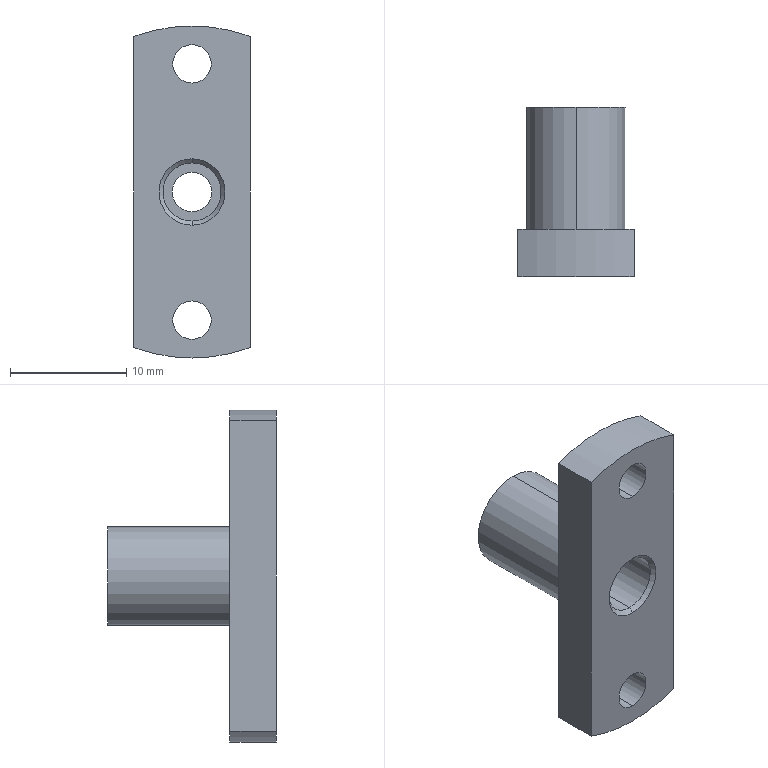Part | NX | features BREP 1 | 1 solid | 23 faces | box 10 x 14.5 x 28.5 mm | volume 1361 mm3 | cylinder 13 | plane 6 | cone 4 | commonest cylinder face diameters 3.3 x4 28.5 x3 3.4 x2 5 x2 8.5 x2
STEP:
#1=CARTESIAN_POINT('',(0.,0.35,2.5));
#2=VERTEX_POINT('',#1);
#3=CARTESIAN_POINT('',(0.,0.,2.85));
#4=VERTEX_POINT('',#3);
#5=CARTESIAN_POINT('',(0.,0.35,2.5));
#6=DIRECTION('',(0.,-0.7071,0.7071));
#7=VECTOR('',#6,1000.);
#8=LINE('',#5,#7);
#9=EDGE_CURVE('',#2,#4,#8,.T.);
#10=ORIENTED_EDGE('',*,*,#9,.F.);
#11=CARTESIAN_POINT('',(0.,0.35,-2.5));
#12=VERTEX_POINT('',#11);
#13=CARTESIAN_POINT('',(0.,0.35,0.));
#14=DIRECTION('',(0.,-1.,0.));
#15=DIRECTION('',(0.,0.,1.));
#16=AXIS2_PLACEMENT_3D('',#13,#14,#15);
#17=CIRCLE('',#16,2.5);
#18=EDGE_CURVE('',#12,#2,#17,.T.);
#19=ORIENTED_EDGE('',*,*,#18,.F.);
#20=CARTESIAN_POINT('',(0.,0.,-2.85));
#21=VERTEX_POINT('',#20);
#22=CARTESIAN_POINT('',(0.,0.35,-2.5));
#23=DIRECTION('',(0.,-0.7071,-0.7071));
#24=VECTOR('',#23,1000.);
#25=LINE('',#22,#24);
#26=EDGE_CURVE('',#12,#21,#25,.T.);
#27=ORIENTED_EDGE('',*,*,#26,.T.);
#28=CARTESIAN_POINT('',(0.,0.,0.));
#29=DIRECTION('',(0.,1.,0.));
#30=DIRECTION('',(0.,0.,1.));
#31=AXIS2_PLACEMENT_3D('',#28,#29,#30);
#32=CIRCLE('',#31,2.85);
#33=EDGE_CURVE('',#4,#21,#32,.T.);
#34=ORIENTED_EDGE('',*,*,#33,.F.);
#35=EDGE_LOOP('',(#10,#19,#27,#34));
#36=FACE_BOUND('',#35,.T.);
#37=CARTESIAN_POINT('',(0.,0.35,0.));
#38=DIRECTION('',(0.,-1.,0.));
#39=DIRECTION('',(0.,0.,-1.));
#40=AXIS2_PLACEMENT_3D('',#37,#38,#39);
#41=CONICAL_SURFACE('',#40,2.5,0.7854);
#42=ADVANCED_FACE('',(#36),#41,.F.);
#43=CARTESIAN_POINT('',(0.,14.5,-3.5));
#44=VERTEX_POINT('',#43);
#45=CARTESIAN_POINT('',(0.,12.7,-1.7));
#46=VERTEX_POINT('',#45);
#47=CARTESIAN_POINT('',(0.,14.5,-3.5));
#48=DIRECTION('',(0.,0.7071,-0.7071));
#49=VECTOR('',#48,1000.);
#50=LINE('',#47,#49);
#51=EDGE_CURVE('',#44,#46,#50,.F.);
#52=ORIENTED_EDGE('',*,*,#51,.T.);
#53=CARTESIAN_POINT('',(0.,12.7,1.7));
#54=VERTEX_POINT('',#53);
#55=CARTESIAN_POINT('',(0.,12.7,0.));
#56=DIRECTION('',(0.,1.,0.));
#57=DIRECTION('',(0.,0.,1.));
#58=AXIS2_PLACEMENT_3D('',#55,#56,#57);
#59=CIRCLE('',#58,1.7);
#60=EDGE_CURVE('',#54,#46,#59,.T.);
#61=ORIENTED_EDGE('',*,*,#60,.F.);
#62=CARTESIAN_POINT('',(0.,14.5,3.5));
#63=VERTEX_POINT('',#62);
#64=CARTESIAN_POINT('',(0.,14.5,3.5));
#65=DIRECTION('',(0.,0.7071,0.7071));
#66=VECTOR('',#65,1000.);
#67=LINE('',#64,#66);
#68=EDGE_CURVE('',#63,#54,#67,.F.);
#69=ORIENTED_EDGE('',*,*,#68,.F.);
#70=CARTESIAN_POINT('',(0.,14.5,0.));
#71=DIRECTION('',(0.,1.,0.));
#72=DIRECTION('',(0.,0.,1.));
#73=AXIS2_PLACEMENT_3D('',#70,#71,#72);
#74=CIRCLE('',#73,3.5);
#75=EDGE_CURVE('',#63,#44,#74,.T.);
#76=ORIENTED_EDGE('',*,*,#75,.T.);
#77=EDGE_LOOP('',(#52,#61,#69,#76));
#78=FACE_BOUND('',#77,.T.);
#79=CARTESIAN_POINT('',(0.,14.5,0.));
#80=DIRECTION('',(0.,1.,0.));
#81=DIRECTION('',(0.,0.,1.));
#82=AXIS2_PLACEMENT_3D('',#79,#80,#81);
#83=CONICAL_SURFACE('',#82,3.5,0.7854);
#84=ADVANCED_FACE('',(#78),#83,.F.);
#85=CARTESIAN_POINT('',(0.,12.,-1.7));
#86=VERTEX_POINT('',#85);
#87=CARTESIAN_POINT('',(0.,14.5,-1.7));
#88=DIRECTION('',(0.,1.,0.));
#89=VECTOR('',#88,1000.);
#90=LINE('',#87,#89);
#91=EDGE_CURVE('',#46,#86,#90,.F.);
#92=ORIENTED_EDGE('',*,*,#91,.T.);
#93=CARTESIAN_POINT('',(0.,12.,1.7));
#94=VERTEX_POINT('',#93);
#95=CARTESIAN_POINT('',(0.,12.,0.));
#96=DIRECTION('',(0.,1.,0.));
#97=DIRECTION('',(0.,0.,1.));
#98=AXIS2_PLACEMENT_3D('',#95,#96,#97);
#99=CIRCLE('',#98,1.7);
#100=EDGE_CURVE('',#94,#86,#99,.T.);
#101=ORIENTED_EDGE('',*,*,#100,.F.);
#102=CARTESIAN_POINT('',(0.,14.5,1.7));
#103=DIRECTION('',(0.,1.,0.));
#104=VECTOR('',#103,1000.);
#105=LINE('',#102,#104);
#106=EDGE_CURVE('',#54,#94,#105,.F.);
#107=ORIENTED_EDGE('',*,*,#106,.F.);
#108=ORIENTED_EDGE('',*,*,#60,.T.);
#109=EDGE_LOOP('',(#92,#101,#107,#108));
#110=FACE_BOUND('',#109,.T.);
#111=CARTESIAN_POINT('',(0.,14.5,0.));
#112=DIRECTION('',(0.,1.,0.));
#113=DIRECTION('',(0.,0.,1.));
#114=AXIS2_PLACEMENT_3D('',#111,#112,#113);
#115=CYLINDRICAL_SURFACE('',#114,1.7);
#116=ADVANCED_FACE('',(#110),#115,.F.);
#117=CARTESIAN_POINT('',(0.,4.,-12.65));
#118=VERTEX_POINT('',#117);
#119=CARTESIAN_POINT('',(0.,0.,-12.65));
#120=VERTEX_POINT('',#119);
#121=CARTESIAN_POINT('',(0.,4.,-12.65));
#122=DIRECTION('',(0.,1.,0.));
#123=VECTOR('',#122,1000.);
#124=LINE('',#121,#123);
#125=EDGE_CURVE('',#118,#120,#124,.F.);
#126=ORIENTED_EDGE('',*,*,#125,.T.);
#127=CARTESIAN_POINT('',(0.,0.,-9.35));
#128=VERTEX_POINT('',#127);
#129=CARTESIAN_POINT('',(0.,0.,-11.));
#130=DIRECTION('',(0.,1.,0.));
#131=DIRECTION('',(0.,0.,1.));
#132=AXIS2_PLACEMENT_3D('',#129,#130,#131);
#133=CIRCLE('',#132,1.65);
#134=EDGE_CURVE('',#128,#120,#133,.T.);
#135=ORIENTED_EDGE('',*,*,#134,.F.);
#136=CARTESIAN_POINT('',(0.,4.,-9.35));
#137=VERTEX_POINT('',#136);
#138=CARTESIAN_POINT('',(0.,4.,-9.35));
#139=DIRECTION('',(0.,1.,0.));
#140=VECTOR('',#139,1000.);
#141=LINE('',#138,#140);
#142=EDGE_CURVE('',#137,#128,#141,.F.);
#143=ORIENTED_EDGE('',*,*,#142,.F.);
#144=CARTESIAN_POINT('',(0.,4.,-11.));
#145=DIRECTION('',(0.,1.,0.));
#146=DIRECTION('',(0.,0.,1.));
#147=AXIS2_PLACEMENT_3D('',#144,#145,#146);
#148=CIRCLE('',#147,1.65);
#149=EDGE_CURVE('',#137,#118,#148,.T.);
#150=ORIENTED_EDGE('',*,*,#149,.T.);
#151=EDGE_LOOP('',(#126,#135,#143,#150));
#152=FACE_BOUND('',#151,.T.);
#153=CARTESIAN_POINT('',(0.,4.,-11.));
#154=DIRECTION('',(0.,1.,0.));
#155=DIRECTION('',(0.,0.,1.));
#156=AXIS2_PLACEMENT_3D('',#153,#154,#155);
#157=CYLINDRICAL_SURFACE('',#156,1.65);
#158=ADVANCED_FACE('',(#152),#157,.F.);
#159=CARTESIAN_POINT('',(0.,4.,9.35));
#160=VERTEX_POINT('',#159);
#161=CARTESIAN_POINT('',(0.,0.,9.35));
#162=VERTEX_POINT('',#161);
#163=CARTESIAN_POINT('',(0.,4.,9.35));
#164=DIRECTION('',(0.,1.,0.));
#165=VECTOR('',#164,1000.);
#166=LINE('',#163,#165);
#167=EDGE_CURVE('',#160,#162,#166,.F.);
#168=ORIENTED_EDGE('',*,*,#167,.T.);
#169=CARTESIAN_POINT('',(0.,0.,12.65));
#170=VERTEX_POINT('',#169);
#171=CARTESIAN_POINT('',(0.,0.,11.));
#172=DIRECTION('',(0.,1.,0.));
#173=DIRECTION('',(0.,0.,1.));
#174=AXIS2_PLACEMENT_3D('',#171,#172,#173);
#175=CIRCLE('',#174,1.65);
#176=EDGE_CURVE('',#170,#162,#175,.T.);
#177=ORIENTED_EDGE('',*,*,#176,.F.);
#178=CARTESIAN_POINT('',(0.,4.,12.65));
#179=VERTEX_POINT('',#178);
#180=CARTESIAN_POINT('',(0.,4.,12.65));
#181=DIRECTION('',(0.,1.,0.));
#182=VECTOR('',#181,1000.);
#183=LINE('',#180,#182);
#184=EDGE_CURVE('',#179,#170,#183,.F.);
#185=ORIENTED_EDGE('',*,*,#184,.F.);
#186=CARTESIAN_POINT('',(0.,4.,11.));
#187=DIRECTION('',(0.,1.,0.));
#188=DIRECTION('',(0.,0.,1.));
#189=AXIS2_PLACEMENT_3D('',#186,#187,#188);
#190=CIRCLE('',#189,1.65);
#191=EDGE_CURVE('',#179,#160,#190,.T.);
#192=ORIENTED_EDGE('',*,*,#191,.T.);
#193=EDGE_LOOP('',(#168,#177,#185,#192));
#194=FACE_BOUND('',#193,.T.);
#195=CARTESIAN_POINT('',(0.,4.,11.));
#196=DIRECTION('',(0.,1.,0.));
#197=DIRECTION('',(0.,0.,1.));
#198=AXIS2_PLACEMENT_3D('',#195,#196,#197);
#199=CYLINDRICAL_SURFACE('',#198,1.65);
#200=ADVANCED_FACE('',(#194),#199,.F.);
#201=CARTESIAN_POINT('',(-5.,0.,13.344));
#202=VERTEX_POINT('',#201);
#203=CARTESIAN_POINT('',(-5.,4.,13.344));
#204=VERTEX_POINT('',#203);
#205=CARTESIAN_POINT('',(-5.,-1.,13.344));
#206=DIRECTION('',(0.,1.,0.));
#207=VECTOR('',#206,1000.);
#208=LINE('',#205,#207);
#209=EDGE_CURVE('',#202,#204,#208,.T.);
#210=ORIENTED_EDGE('',*,*,#209,.T.);
#211=CARTESIAN_POINT('',(-5.,4.,-13.344));
#212=VERTEX_POINT('',#211);
#213=CARTESIAN_POINT('',(-5.,4.,13.344));
#214=DIRECTION('',(0.,0.,-1.));
#215=VECTOR('',#214,1000.);
#216=LINE('',#213,#215);
#217=EDGE_CURVE('',#204,#212,#216,.T.);
#218=ORIENTED_EDGE('',*,*,#217,.T.);
#219=CARTESIAN_POINT('',(-5.,0.,-13.344));
#220=VERTEX_POINT('',#219);
#221=CARTESIAN_POINT('',(-5.,-1.,-13.344));
#222=DIRECTION('',(0.,1.,0.));
#223=VECTOR('',#222,1000.);
#224=LINE('',#221,#223);
#225=EDGE_CURVE('',#220,#212,#224,.T.);
#226=ORIENTED_EDGE('',*,*,#225,.F.);
#227=CARTESIAN_POINT('',(-5.,0.,0.));
#228=DIRECTION('',(0.,0.,-1.));
#229=VECTOR('',#228,1000.);
#230=LINE('',#227,#229);
#231=EDGE_CURVE('',#202,#220,#230,.T.);
#232=ORIENTED_EDGE('',*,*,#231,.F.);
#233=EDGE_LOOP('',(#210,#218,#226,#232));
#234=FACE_BOUND('',#233,.T.);
#235=CARTESIAN_POINT('',(-5.,-1.,13.344));
#236=DIRECTION('',(1.,0.,0.));
#237=DIRECTION('',(0.,0.,-1.));
#238=AXIS2_PLACEMENT_3D('',#235,#236,#237);
#239=PLANE('',#238);
#240=ADVANCED_FACE('',(#234),#239,.F.);
#241=CARTESIAN_POINT('',(5.,0.,-13.344));
#242=VERTEX_POINT('',#241);
#243=CARTESIAN_POINT('',(5.,4.,-13.344));
#244=VERTEX_POINT('',#243);
#245=CARTESIAN_POINT('',(5.,-1.,-13.344));
#246=DIRECTION('',(0.,1.,0.));
#247=VECTOR('',#246,1000.);
#248=LINE('',#245,#247);
#249=EDGE_CURVE('',#242,#244,#248,.T.);
#250=ORIENTED_EDGE('',*,*,#249,.T.);
#251=CARTESIAN_POINT('',(5.,4.,13.344));
#252=VERTEX_POINT('',#251);
#253=CARTESIAN_POINT('',(5.,4.,13.344));
#254=DIRECTION('',(0.,0.,1.));
#255=VECTOR('',#254,1000.);
#256=LINE('',#253,#255);
#257=EDGE_CURVE('',#244,#252,#256,.T.);
#258=ORIENTED_EDGE('',*,*,#257,.T.);
#259=CARTESIAN_POINT('',(5.,0.,13.344));
#260=VERTEX_POINT('',#259);
#261=CARTESIAN_POINT('',(5.,-1.,13.344));
#262=DIRECTION('',(0.,1.,0.));
#263=VECTOR('',#262,1000.);
#264=LINE('',#261,#263);
#265=EDGE_CURVE('',#260,#252,#264,.T.);
#266=ORIENTED_EDGE('',*,*,#265,.F.);
#267=CARTESIAN_POINT('',(5.,0.,0.));
#268=DIRECTION('',(0.,0.,1.));
#269=VECTOR('',#268,1000.);
#270=LINE('',#267,#269);
#271=EDGE_CURVE('',#242,#260,#270,.T.);
#272=ORIENTED_EDGE('',*,*,#271,.F.);
#273=EDGE_LOOP('',(#250,#258,#266,#272));
#274=FACE_BOUND('',#273,.T.);
#275=CARTESIAN_POINT('',(5.,-1.,13.344));
#276=DIRECTION('',(-1.,0.,0.));
#277=DIRECTION('',(0.,0.,1.));
#278=AXIS2_PLACEMENT_3D('',#275,#276,#277);
#279=PLANE('',#278);
#280=ADVANCED_FACE('',(#274),#279,.F.);
#281=CARTESIAN_POINT('',(0.,14.5,-4.25));
#282=VERTEX_POINT('',#281);
#283=CARTESIAN_POINT('',(0.,14.5,4.25));
#284=VERTEX_POINT('',#283);
#285=CARTESIAN_POINT('',(0.,14.5,0.));
#286=DIRECTION('',(0.,1.,0.));
#287=DIRECTION('',(0.,0.,1.));
#288=AXIS2_PLACEMENT_3D('',#285,#286,#287);
#289=CIRCLE('',#288,4.25);
#290=EDGE_CURVE('',#282,#284,#289,.T.);
#291=ORIENTED_EDGE('',*,*,#290,.T.);
#292=CARTESIAN_POINT('',(0.,14.5,0.));
#293=DIRECTION('',(0.,1.,0.));
#294=DIRECTION('',(0.,0.,1.));
#295=AXIS2_PLACEMENT_3D('',#292,#293,#294);
#296=CIRCLE('',#295,4.25);
#297=EDGE_CURVE('',#284,#282,#296,.T.);
#298=ORIENTED_EDGE('',*,*,#297,.T.);
#299=EDGE_LOOP('',(#291,#298));
#300=FACE_BOUND('',#299,.T.);
#301=ORIENTED_EDGE('',*,*,#75,.F.);
#302=CARTESIAN_POINT('',(0.,14.5,0.));
#303=DIRECTION('',(0.,1.,0.));
#304=DIRECTION('',(0.,0.,1.));
#305=AXIS2_PLACEMENT_3D('',#302,#303,#304);
#306=CIRCLE('',#305,3.5);
#307=EDGE_CURVE('',#44,#63,#306,.T.);
#308=ORIENTED_EDGE('',*,*,#307,.F.);
#309=EDGE_LOOP('',(#301,#308));
#310=FACE_BOUND('',#309,.T.);
#311=CARTESIAN_POINT('',(0.,14.5,0.));
#312=DIRECTION('',(0.,1.,0.));
#313=DIRECTION('',(0.,0.,1.));
#314=AXIS2_PLACEMENT_3D('',#311,#312,#313);
#315=PLANE('',#314);
#316=ADVANCED_FACE('',(#300,#310),#315,.T.);
#317=CARTESIAN_POINT('',(0.,12.,-2.5));
#318=VERTEX_POINT('',#317);
#319=CARTESIAN_POINT('',(0.,12.,2.5));
#320=VERTEX_POINT('',#319);
#321=CARTESIAN_POINT('',(0.,12.,0.));
#322=DIRECTION('',(0.,-1.,0.));
#323=DIRECTION('',(0.,0.,-1.));
#324=AXIS2_PLACEMENT_3D('',#321,#322,#323);
#325=CIRCLE('',#324,2.5);
#326=EDGE_CURVE('',#318,#320,#325,.T.);
#327=ORIENTED_EDGE('',*,*,#326,.T.);
#328=CARTESIAN_POINT('',(0.,12.,0.));
#329=DIRECTION('',(0.,-1.,0.));
#330=DIRECTION('',(0.,0.,-1.));
#331=AXIS2_PLACEMENT_3D('',#328,#329,#330);
#332=CIRCLE('',#331,2.5);
#333=EDGE_CURVE('',#320,#318,#332,.T.);
#334=ORIENTED_EDGE('',*,*,#333,.T.);
#335=EDGE_LOOP('',(#327,#334));
#336=FACE_BOUND('',#335,.T.);
#337=ORIENTED_EDGE('',*,*,#100,.T.);
#338=CARTESIAN_POINT('',(0.,12.,0.));
#339=DIRECTION('',(0.,1.,0.));
#340=DIRECTION('',(0.,0.,1.));
#341=AXIS2_PLACEMENT_3D('',#338,#339,#340);
#342=CIRCLE('',#341,1.7);
#343=EDGE_CURVE('',#86,#94,#342,.T.);
#344=ORIENTED_EDGE('',*,*,#343,.T.);
#345=EDGE_LOOP('',(#337,#344));
#346=FACE_BOUND('',#345,.T.);
#347=CARTESIAN_POINT('',(0.,12.,0.));
#348=DIRECTION('',(0.,1.,0.));
#349=DIRECTION('',(0.,0.,1.));
#350=AXIS2_PLACEMENT_3D('',#347,#348,#349);
#351=PLANE('',#350);
#352=ADVANCED_FACE('',(#336,#346),#351,.F.);
#353=CARTESIAN_POINT('',(0.,4.,4.25));
#354=VERTEX_POINT('',#353);
#355=CARTESIAN_POINT('',(0.,0.,4.25));
#356=DIRECTION('',(0.,-1.,0.));
#357=VECTOR('',#356,1000.);
#358=LINE('',#355,#357);
#359=EDGE_CURVE('',#284,#354,#358,.T.);
#360=ORIENTED_EDGE('',*,*,#359,.F.);
#361=ORIENTED_EDGE('',*,*,#290,.F.);
#362=CARTESIAN_POINT('',(0.,4.,-4.25));
#363=VERTEX_POINT('',#362);
#364=CARTESIAN_POINT('',(0.,0.,-4.25));
#365=DIRECTION('',(0.,-1.,0.));
#366=VECTOR('',#365,1000.);
#367=LINE('',#364,#366);
#368=EDGE_CURVE('',#282,#363,#367,.T.);
#369=ORIENTED_EDGE('',*,*,#368,.T.);
#370=CARTESIAN_POINT('',(0.,4.,0.));
#371=DIRECTION('',(0.,-1.,0.));
#372=DIRECTION('',(0.,0.,-1.));
#373=AXIS2_PLACEMENT_3D('',#370,#371,#372);
#374=CIRCLE('',#373,4.25);
#375=EDGE_CURVE('',#354,#363,#374,.T.);
#376=ORIENTED_EDGE('',*,*,#375,.F.);
#377=EDGE_LOOP('',(#360,#361,#369,#376));
#378=FACE_BOUND('',#377,.T.);
#379=CARTESIAN_POINT('',(0.,0.,0.));
#380=DIRECTION('',(0.,-1.,0.));
#381=DIRECTION('',(0.,0.,-1.));
#382=AXIS2_PLACEMENT_3D('',#379,#380,#381);
#383=CYLINDRICAL_SURFACE('',#382,4.25);
#384=ADVANCED_FACE('',(#378),#383,.T.);
#385=CARTESIAN_POINT('',(0.,4.,0.));
#386=DIRECTION('',(0.,-1.,0.));
#387=DIRECTION('',(0.,0.,-1.));
#388=AXIS2_PLACEMENT_3D('',#385,#386,#387);
#389=CIRCLE('',#388,4.25);
#390=EDGE_CURVE('',#363,#354,#389,.T.);
#391=ORIENTED_EDGE('',*,*,#390,.T.);
#392=ORIENTED_EDGE('',*,*,#375,.T.);
#393=EDGE_LOOP('',(#391,#392));
#394=FACE_BOUND('',#393,.T.);
#395=CARTESIAN_POINT('',(0.,4.,-14.25));
#396=VERTEX_POINT('',#395);
#397=CARTESIAN_POINT('',(0.,4.,0.));
#398=DIRECTION('',(0.,-1.,0.));
#399=DIRECTION('',(0.,0.,-1.));
#400=AXIS2_PLACEMENT_3D('',#397,#398,#399);
#401=CIRCLE('',#400,14.25);
#402=EDGE_CURVE('',#212,#396,#401,.T.);
#403=ORIENTED_EDGE('',*,*,#402,.F.);
#404=ORIENTED_EDGE('',*,*,#217,.F.);
#405=CARTESIAN_POINT('',(0.,4.,0.));
#406=DIRECTION('',(0.,-1.,0.));
#407=DIRECTION('',(0.,0.,-1.));
#408=AXIS2_PLACEMENT_3D('',#405,#406,#407);
#409=CIRCLE('',#408,14.25);
#410=EDGE_CURVE('',#252,#204,#409,.T.);
#411=ORIENTED_EDGE('',*,*,#410,.F.);
#412=ORIENTED_EDGE('',*,*,#257,.F.);
#413=CARTESIAN_POINT('',(0.,4.,0.));
#414=DIRECTION('',(0.,-1.,0.));
#415=DIRECTION('',(0.,0.,-1.));
#416=AXIS2_PLACEMENT_3D('',#413,#414,#415);
#417=CIRCLE('',#416,14.25);
#418=EDGE_CURVE('',#396,#244,#417,.T.);
#419=ORIENTED_EDGE('',*,*,#418,.F.);
#420=EDGE_LOOP('',(#403,#404,#411,#412,#419));
#421=FACE_BOUND('',#420,.T.);
#422=ORIENTED_EDGE('',*,*,#191,.F.);
#423=CARTESIAN_POINT('',(0.,4.,11.));
#424=DIRECTION('',(0.,1.,0.));
#425=DIRECTION('',(0.,0.,1.));
#426=AXIS2_PLACEMENT_3D('',#423,#424,#425);
#427=CIRCLE('',#426,1.65);
#428=EDGE_CURVE('',#160,#179,#427,.T.);
#429=ORIENTED_EDGE('',*,*,#428,.F.);
#430=EDGE_LOOP('',(#422,#429));
#431=FACE_BOUND('',#430,.T.);
#432=ORIENTED_EDGE('',*,*,#149,.F.);
#433=CARTESIAN_POINT('',(0.,4.,-11.));
#434=DIRECTION('',(0.,1.,0.));
#435=DIRECTION('',(0.,0.,1.));
#436=AXIS2_PLACEMENT_3D('',#433,#434,#435);
#437=CIRCLE('',#436,1.65);
#438=EDGE_CURVE('',#118,#137,#437,.T.);
#439=ORIENTED_EDGE('',*,*,#438,.F.);
#440=EDGE_LOOP('',(#432,#439));
#441=FACE_BOUND('',#440,.T.);
#442=CARTESIAN_POINT('',(-14.25,4.,0.));
#443=DIRECTION('',(0.,-1.,0.));
#444=DIRECTION('',(0.,0.,-1.));
#445=AXIS2_PLACEMENT_3D('',#442,#443,#444);
#446=PLANE('',#445);
#447=ADVANCED_FACE('',(#394,#421,#431,#441),#446,.F.);
#448=CARTESIAN_POINT('',(0.,0.,-14.25));
#449=VERTEX_POINT('',#448);
#450=CARTESIAN_POINT('',(0.,0.,-14.25));
#451=DIRECTION('',(0.,-1.,0.));
#452=VECTOR('',#451,1000.);
#453=LINE('',#450,#452);
#454=EDGE_CURVE('',#396,#449,#453,.T.);
#455=ORIENTED_EDGE('',*,*,#454,.F.);
#456=ORIENTED_EDGE('',*,*,#418,.T.);
#457=ORIENTED_EDGE('',*,*,#249,.F.);
#458=CARTESIAN_POINT('',(0.,0.,0.));
#459=DIRECTION('',(0.,-1.,0.));
#460=DIRECTION('',(0.,0.,-1.));
#461=AXIS2_PLACEMENT_3D('',#458,#459,#460);
#462=CIRCLE('',#461,14.25);
#463=EDGE_CURVE('',#449,#242,#462,.T.);
#464=ORIENTED_EDGE('',*,*,#463,.F.);
#465=EDGE_LOOP('',(#455,#456,#457,#464));
#466=FACE_BOUND('',#465,.T.);
#467=CARTESIAN_POINT('',(0.,0.,0.));
#468=DIRECTION('',(0.,-1.,0.));
#469=DIRECTION('',(0.,0.,-1.));
#470=AXIS2_PLACEMENT_3D('',#467,#468,#469);
#471=CYLINDRICAL_SURFACE('',#470,14.25);
#472=ADVANCED_FACE('',(#466),#471,.T.);
#473=CARTESIAN_POINT('',(0.,0.,0.));
#474=DIRECTION('',(0.,-1.,0.));
#475=DIRECTION('',(0.,0.,-1.));
#476=AXIS2_PLACEMENT_3D('',#473,#474,#475);
#477=CIRCLE('',#476,14.25);
#478=EDGE_CURVE('',#260,#202,#477,.T.);
#479=ORIENTED_EDGE('',*,*,#478,.T.);
#480=ORIENTED_EDGE('',*,*,#231,.T.);
#481=CARTESIAN_POINT('',(0.,0.,0.));
#482=DIRECTION('',(0.,-1.,0.));
#483=DIRECTION('',(0.,0.,-1.));
#484=AXIS2_PLACEMENT_3D('',#481,#482,#483);
#485=CIRCLE('',#484,14.25);
#486=EDGE_CURVE('',#220,#449,#485,.T.);
#487=ORIENTED_EDGE('',*,*,#486,.T.);
#488=ORIENTED_EDGE('',*,*,#463,.T.);
#489=ORIENTED_EDGE('',*,*,#271,.T.);
#490=EDGE_LOOP('',(#479,#480,#487,#488,#489));
#491=FACE_BOUND('',#490,.T.);
#492=ORIENTED_EDGE('',*,*,#176,.T.);
#493=CARTESIAN_POINT('',(0.,0.,11.));
#494=DIRECTION('',(0.,1.,0.));
#495=DIRECTION('',(0.,0.,1.));
#496=AXIS2_PLACEMENT_3D('',#493,#494,#495);
#497=CIRCLE('',#496,1.65);
#498=EDGE_CURVE('',#162,#170,#497,.T.);
#499=ORIENTED_EDGE('',*,*,#498,.T.);
#500=EDGE_LOOP('',(#492,#499));
#501=FACE_BOUND('',#500,.T.);
#502=ORIENTED_EDGE('',*,*,#134,.T.);
#503=CARTESIAN_POINT('',(0.,0.,-11.));
#504=DIRECTION('',(0.,1.,0.));
#505=DIRECTION('',(0.,0.,1.));
#506=AXIS2_PLACEMENT_3D('',#503,#504,#505);
#507=CIRCLE('',#506,1.65);
#508=EDGE_CURVE('',#120,#128,#507,.T.);
#509=ORIENTED_EDGE('',*,*,#508,.T.);
#510=EDGE_LOOP('',(#502,#509));
#511=FACE_BOUND('',#510,.T.);
#512=CARTESIAN_POINT('',(0.,0.,0.));
#513=DIRECTION('',(0.,1.,0.));
#514=DIRECTION('',(0.,0.,1.));
#515=AXIS2_PLACEMENT_3D('',#512,#513,#514);
#516=CIRCLE('',#515,2.85);
#517=EDGE_CURVE('',#21,#4,#516,.T.);
#518=ORIENTED_EDGE('',*,*,#517,.T.);
#519=ORIENTED_EDGE('',*,*,#33,.T.);
#520=EDGE_LOOP('',(#518,#519));
#521=FACE_BOUND('',#520,.T.);
#522=CARTESIAN_POINT('',(-2.5,0.,0.));
#523=DIRECTION('',(0.,1.,0.));
#524=DIRECTION('',(0.,0.,1.));
#525=AXIS2_PLACEMENT_3D('',#522,#523,#524);
#526=PLANE('',#525);
#527=ADVANCED_FACE('',(#491,#501,#511,#521),#526,.F.);
#528=CARTESIAN_POINT('',(0.,0.,2.5));
#529=DIRECTION('',(0.,-1.,0.));
#530=VECTOR('',#529,1000.);
#531=LINE('',#528,#530);
#532=EDGE_CURVE('',#320,#2,#531,.T.);
#533=ORIENTED_EDGE('',*,*,#532,.F.);
#534=ORIENTED_EDGE('',*,*,#326,.F.);
#535=CARTESIAN_POINT('',(0.,0.,-2.5));
#536=DIRECTION('',(0.,-1.,0.));
#537=VECTOR('',#536,1000.);
#538=LINE('',#535,#537);
#539=EDGE_CURVE('',#318,#12,#538,.T.);
#540=ORIENTED_EDGE('',*,*,#539,.T.);
#541=ORIENTED_EDGE('',*,*,#18,.T.);
#542=EDGE_LOOP('',(#533,#534,#540,#541));
#543=FACE_BOUND('',#542,.T.);
#544=CARTESIAN_POINT('',(0.,0.,0.));
#545=DIRECTION('',(0.,-1.,0.));
#546=DIRECTION('',(0.,0.,-1.));
#547=AXIS2_PLACEMENT_3D('',#544,#545,#546);
#548=CYLINDRICAL_SURFACE('',#547,2.5);
#549=ADVANCED_FACE('',(#543),#548,.F.);
#550=ORIENTED_EDGE('',*,*,#410,.T.);
#551=ORIENTED_EDGE('',*,*,#209,.F.);
#552=ORIENTED_EDGE('',*,*,#478,.F.);
#553=ORIENTED_EDGE('',*,*,#265,.T.);
#554=EDGE_LOOP('',(#550,#551,#552,#553));
#555=FACE_BOUND('',#554,.T.);
#556=CARTESIAN_POINT('',(0.,0.,0.));
#557=DIRECTION('',(0.,-1.,0.));
#558=DIRECTION('',(0.,0.,-1.));
#559=AXIS2_PLACEMENT_3D('',#556,#557,#558);
#560=CYLINDRICAL_SURFACE('',#559,14.25);
#561=ADVANCED_FACE('',(#555),#560,.T.);
#562=ORIENTED_EDGE('',*,*,#333,.F.);
#563=ORIENTED_EDGE('',*,*,#532,.T.);
#564=CARTESIAN_POINT('',(0.,0.35,0.));
#565=DIRECTION('',(0.,-1.,0.));
#566=DIRECTION('',(0.,0.,1.));
#567=AXIS2_PLACEMENT_3D('',#564,#565,#566);
#568=CIRCLE('',#567,2.5);
#569=EDGE_CURVE('',#2,#12,#568,.T.);
#570=ORIENTED_EDGE('',*,*,#569,.T.);
#571=ORIENTED_EDGE('',*,*,#539,.F.);
#572=EDGE_LOOP('',(#562,#563,#570,#571));
#573=FACE_BOUND('',#572,.T.);
#574=CARTESIAN_POINT('',(0.,0.,0.));
#575=DIRECTION('',(0.,-1.,0.));
#576=DIRECTION('',(0.,0.,-1.));
#577=AXIS2_PLACEMENT_3D('',#574,#575,#576);
#578=CYLINDRICAL_SURFACE('',#577,2.5);
#579=ADVANCED_FACE('',(#573),#578,.F.);
#580=ORIENTED_EDGE('',*,*,#402,.T.);
#581=ORIENTED_EDGE('',*,*,#454,.T.);
#582=ORIENTED_EDGE('',*,*,#486,.F.);
#583=ORIENTED_EDGE('',*,*,#225,.T.);
#584=EDGE_LOOP('',(#580,#581,#582,#583));
#585=FACE_BOUND('',#584,.T.);
#586=CARTESIAN_POINT('',(0.,0.,0.));
#587=DIRECTION('',(0.,-1.,0.));
#588=DIRECTION('',(0.,0.,-1.));
#589=AXIS2_PLACEMENT_3D('',#586,#587,#588);
#590=CYLINDRICAL_SURFACE('',#589,14.25);
#591=ADVANCED_FACE('',(#585),#590,.T.);
#592=ORIENTED_EDGE('',*,*,#297,.F.);
#593=ORIENTED_EDGE('',*,*,#359,.T.);
#594=ORIENTED_EDGE('',*,*,#390,.F.);
#595=ORIENTED_EDGE('',*,*,#368,.F.);
#596=EDGE_LOOP('',(#592,#593,#594,#595));
#597=FACE_BOUND('',#596,.T.);
#598=CARTESIAN_POINT('',(0.,0.,0.));
#599=DIRECTION('',(0.,-1.,0.));
#600=DIRECTION('',(0.,0.,-1.));
#601=AXIS2_PLACEMENT_3D('',#598,#599,#600);
#602=CYLINDRICAL_SURFACE('',#601,4.25);
#603=ADVANCED_FACE('',(#597),#602,.T.);
#604=ORIENTED_EDGE('',*,*,#498,.F.);
#605=ORIENTED_EDGE('',*,*,#167,.F.);
#606=ORIENTED_EDGE('',*,*,#428,.T.);
#607=ORIENTED_EDGE('',*,*,#184,.T.);
#608=EDGE_LOOP('',(#604,#605,#606,#607));
#609=FACE_BOUND('',#608,.T.);
#610=CARTESIAN_POINT('',(0.,4.,11.));
#611=DIRECTION('',(0.,1.,0.));
#612=DIRECTION('',(0.,0.,1.));
#613=AXIS2_PLACEMENT_3D('',#610,#611,#612);
#614=CYLINDRICAL_SURFACE('',#613,1.65);
#615=ADVANCED_FACE('',(#609),#614,.F.);
#616=ORIENTED_EDGE('',*,*,#508,.F.);
#617=ORIENTED_EDGE('',*,*,#125,.F.);
#618=ORIENTED_EDGE('',*,*,#438,.T.);
#619=ORIENTED_EDGE('',*,*,#142,.T.);
#620=EDGE_LOOP('',(#616,#617,#618,#619));
#621=FACE_BOUND('',#620,.T.);
#622=CARTESIAN_POINT('',(0.,4.,-11.));
#623=DIRECTION('',(0.,1.,0.));
#624=DIRECTION('',(0.,0.,1.));
#625=AXIS2_PLACEMENT_3D('',#622,#623,#624);
#626=CYLINDRICAL_SURFACE('',#625,1.65);
#627=ADVANCED_FACE('',(#621),#626,.F.);
#628=ORIENTED_EDGE('',*,*,#343,.F.);
#629=ORIENTED_EDGE('',*,*,#91,.F.);
#630=CARTESIAN_POINT('',(0.,12.7,0.));
#631=DIRECTION('',(0.,1.,0.));
#632=DIRECTION('',(0.,0.,1.));
#633=AXIS2_PLACEMENT_3D('',#630,#631,#632);
#634=CIRCLE('',#633,1.7);
#635=EDGE_CURVE('',#46,#54,#634,.T.);
#636=ORIENTED_EDGE('',*,*,#635,.T.);
#637=ORIENTED_EDGE('',*,*,#106,.T.);
#638=EDGE_LOOP('',(#628,#629,#636,#637));
#639=FACE_BOUND('',#638,.T.);
#640=CARTESIAN_POINT('',(0.,14.5,0.));
#641=DIRECTION('',(0.,1.,0.));
#642=DIRECTION('',(0.,0.,1.));
#643=AXIS2_PLACEMENT_3D('',#640,#641,#642);
#644=CYLINDRICAL_SURFACE('',#643,1.7);
#645=ADVANCED_FACE('',(#639),#644,.F.);
#646=ORIENTED_EDGE('',*,*,#635,.F.);
#647=ORIENTED_EDGE('',*,*,#51,.F.);
#648=ORIENTED_EDGE('',*,*,#307,.T.);
#649=ORIENTED_EDGE('',*,*,#68,.T.);
#650=EDGE_LOOP('',(#646,#647,#648,#649));
#651=FACE_BOUND('',#650,.T.);
#652=CARTESIAN_POINT('',(0.,14.5,0.));
#653=DIRECTION('',(0.,1.,0.));
#654=DIRECTION('',(0.,0.,1.));
#655=AXIS2_PLACEMENT_3D('',#652,#653,#654);
#656=CONICAL_SURFACE('',#655,3.5,0.7854);
#657=ADVANCED_FACE('',(#651),#656,.F.);
#658=ORIENTED_EDGE('',*,*,#569,.F.);
#659=ORIENTED_EDGE('',*,*,#9,.T.);
#660=ORIENTED_EDGE('',*,*,#517,.F.);
#661=ORIENTED_EDGE('',*,*,#26,.F.);
#662=EDGE_LOOP('',(#658,#659,#660,#661));
#663=FACE_BOUND('',#662,.T.);
#664=CARTESIAN_POINT('',(0.,0.35,0.));
#665=DIRECTION('',(0.,-1.,0.));
#666=DIRECTION('',(0.,0.,-1.));
#667=AXIS2_PLACEMENT_3D('',#664,#665,#666);
#668=CONICAL_SURFACE('',#667,2.5,0.7854);
#669=ADVANCED_FACE('',(#663),#668,.F.);
#670=CLOSED_SHELL('',(#42,#84,#116,#158,#200,#240,#280,#316,#352,#384,#447,#472,#527,#549,#561,#579,#591,#603,#615,#627,#645,#657,#669));
#671=MANIFOLD_SOLID_BREP('',#670);
#672=(LENGTH_UNIT()NAMED_UNIT(*)SI_UNIT(.MILLI.,.METRE.));
#673=UNCERTAINTY_MEASURE_WITH_UNIT(LENGTH_MEASURE(0.00001),#672,'','');
#674=(NAMED_UNIT(*)PLANE_ANGLE_UNIT()SI_UNIT($,.RADIAN.));
#675=(NAMED_UNIT(*)SI_UNIT($,.STERADIAN.)SOLID_ANGLE_UNIT());
#676=(GEOMETRIC_REPRESENTATION_CONTEXT(3)GLOBAL_UNCERTAINTY_ASSIGNED_CONTEXT((#673))GLOBAL_UNIT_ASSIGNED_CONTEXT((#672,#674,#675))REPRESENTATION_CONTEXT('',''));
#677=ADVANCED_BREP_SHAPE_REPRESENTATION('',(#671),#676);